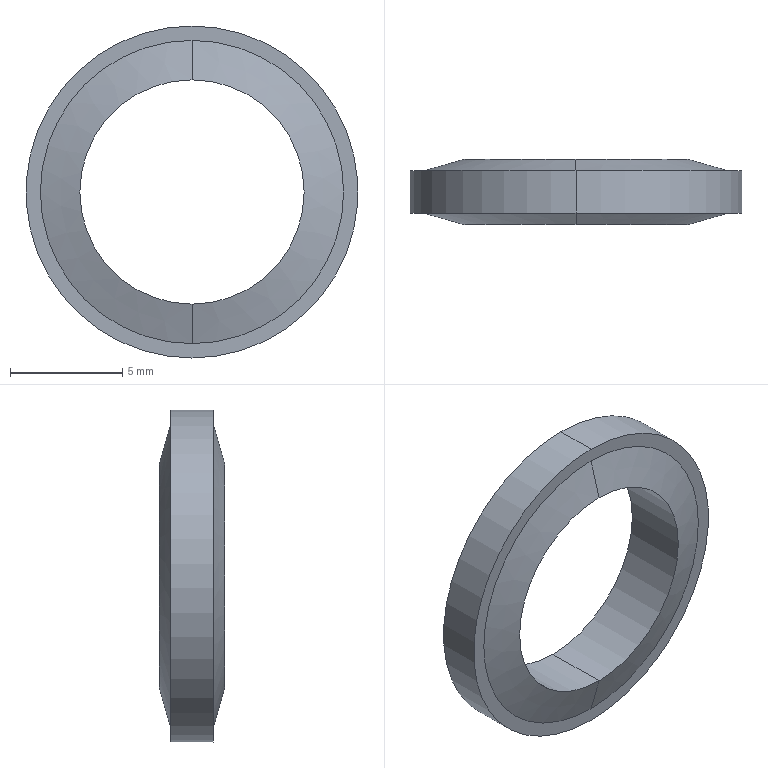Part | SolidWorks | features BaseBody 2 | 2 solids | 14 faces | box 14.8 x 2.9 x 14.8 mm | volume 208.528 mm3 | cylinder 8 | cone 4 | plane 2 | commonest cylinder face diameters 13.52 x4 10 x2 14.8 x2
STEP:
#1=CARTESIAN_POINT('',(0.,1.9,-6.76));
#2=VERTEX_POINT('',#1);
#3=CARTESIAN_POINT('',(0.,0.,-6.76));
#4=VERTEX_POINT('',#3);
#5=CARTESIAN_POINT('',(0.,1.9,-6.76));
#6=DIRECTION('',(0.,-1.,0.));
#7=VECTOR('',#6,1000.);
#8=LINE('',#5,#7);
#9=EDGE_CURVE('',#2,#4,#8,.T.);
#10=ORIENTED_EDGE('',*,*,#9,.T.);
#11=CARTESIAN_POINT('',(0.,0.,6.76));
#12=VERTEX_POINT('',#11);
#13=CARTESIAN_POINT('',(0.,0.,0.));
#14=DIRECTION('',(0.,-1.,0.));
#15=DIRECTION('',(0.,0.,-1.));
#16=AXIS2_PLACEMENT_3D('',#13,#14,#15);
#17=CIRCLE('',#16,6.76);
#18=EDGE_CURVE('',#4,#12,#17,.T.);
#19=ORIENTED_EDGE('',*,*,#18,.T.);
#20=CARTESIAN_POINT('',(0.,1.9,6.76));
#21=VERTEX_POINT('',#20);
#22=CARTESIAN_POINT('',(0.,1.9,6.76));
#23=DIRECTION('',(0.,-1.,0.));
#24=VECTOR('',#23,1000.);
#25=LINE('',#22,#24);
#26=EDGE_CURVE('',#21,#12,#25,.T.);
#27=ORIENTED_EDGE('',*,*,#26,.F.);
#28=CARTESIAN_POINT('',(0.,1.9,0.));
#29=DIRECTION('',(0.,-1.,0.));
#30=DIRECTION('',(0.,0.,-1.));
#31=AXIS2_PLACEMENT_3D('',#28,#29,#30);
#32=CIRCLE('',#31,6.76);
#33=EDGE_CURVE('',#2,#21,#32,.T.);
#34=ORIENTED_EDGE('',*,*,#33,.F.);
#35=EDGE_LOOP('',(#10,#19,#27,#34));
#36=FACE_OUTER_BOUND('',#35,.T.);
#37=CARTESIAN_POINT('',(0.,1.9,0.));
#38=DIRECTION('',(0.,-1.,0.));
#39=DIRECTION('',(0.,0.,1.));
#40=AXIS2_PLACEMENT_3D('',#37,#38,#39);
#41=CYLINDRICAL_SURFACE('',#40,6.76);
#42=ADVANCED_FACE('',(#36),#41,.F.);
#43=CARTESIAN_POINT('',(0.,1.9,-7.4));
#44=VERTEX_POINT('',#43);
#45=CARTESIAN_POINT('',(0.,0.,-7.4));
#46=VERTEX_POINT('',#45);
#47=CARTESIAN_POINT('',(0.,1.9,-7.4));
#48=DIRECTION('',(0.,-1.,0.));
#49=VECTOR('',#48,1000.);
#50=LINE('',#47,#49);
#51=EDGE_CURVE('',#44,#46,#50,.T.);
#52=ORIENTED_EDGE('',*,*,#51,.T.);
#53=CARTESIAN_POINT('',(0.,0.,7.4));
#54=VERTEX_POINT('',#53);
#55=CARTESIAN_POINT('',(0.,0.,0.));
#56=DIRECTION('',(0.,-1.,0.));
#57=DIRECTION('',(0.,0.,-1.));
#58=AXIS2_PLACEMENT_3D('',#55,#56,#57);
#59=CIRCLE('',#58,7.4);
#60=EDGE_CURVE('',#54,#46,#59,.T.);
#61=ORIENTED_EDGE('',*,*,#60,.F.);
#62=CARTESIAN_POINT('',(0.,1.9,7.4));
#63=VERTEX_POINT('',#62);
#64=CARTESIAN_POINT('',(0.,1.9,7.4));
#65=DIRECTION('',(0.,-1.,0.));
#66=VECTOR('',#65,1000.);
#67=LINE('',#64,#66);
#68=EDGE_CURVE('',#63,#54,#67,.T.);
#69=ORIENTED_EDGE('',*,*,#68,.F.);
#70=CARTESIAN_POINT('',(0.,1.9,0.));
#71=DIRECTION('',(0.,-1.,0.));
#72=DIRECTION('',(0.,0.,-1.));
#73=AXIS2_PLACEMENT_3D('',#70,#71,#72);
#74=CIRCLE('',#73,7.4);
#75=EDGE_CURVE('',#63,#44,#74,.T.);
#76=ORIENTED_EDGE('',*,*,#75,.T.);
#77=EDGE_LOOP('',(#52,#61,#69,#76));
#78=FACE_OUTER_BOUND('',#77,.T.);
#79=CARTESIAN_POINT('',(0.,1.9,0.));
#80=DIRECTION('',(0.,-1.,0.));
#81=DIRECTION('',(0.,0.,1.));
#82=AXIS2_PLACEMENT_3D('',#79,#80,#81);
#83=CYLINDRICAL_SURFACE('',#82,7.4);
#84=ADVANCED_FACE('',(#78),#83,.T.);
#85=CARTESIAN_POINT('',(0.,0.,0.));
#86=DIRECTION('',(0.,-1.,0.));
#87=DIRECTION('',(0.,0.,-1.));
#88=AXIS2_PLACEMENT_3D('',#85,#86,#87);
#89=CIRCLE('',#88,6.76);
#90=EDGE_CURVE('',#12,#4,#89,.T.);
#91=ORIENTED_EDGE('',*,*,#90,.F.);
#92=ORIENTED_EDGE('',*,*,#18,.F.);
#93=EDGE_LOOP('',(#91,#92));
#94=FACE_BOUND('',#93,.T.);
#95=ORIENTED_EDGE('',*,*,#60,.T.);
#96=CARTESIAN_POINT('',(0.,0.,0.));
#97=DIRECTION('',(0.,-1.,0.));
#98=DIRECTION('',(0.,0.,-1.));
#99=AXIS2_PLACEMENT_3D('',#96,#97,#98);
#100=CIRCLE('',#99,7.4);
#101=EDGE_CURVE('',#46,#54,#100,.T.);
#102=ORIENTED_EDGE('',*,*,#101,.T.);
#103=EDGE_LOOP('',(#95,#102));
#104=FACE_OUTER_BOUND('',#103,.T.);
#105=CARTESIAN_POINT('',(0.,0.,0.));
#106=DIRECTION('',(0.,1.,0.));
#107=DIRECTION('',(1.,0.,0.));
#108=AXIS2_PLACEMENT_3D('',#105,#106,#107);
#109=PLANE('',#108);
#110=ADVANCED_FACE('',(#94,#104),#109,.F.);
#111=CARTESIAN_POINT('',(0.,1.9,0.));
#112=DIRECTION('',(0.,-1.,0.));
#113=DIRECTION('',(0.,0.,-1.));
#114=AXIS2_PLACEMENT_3D('',#111,#112,#113);
#115=CIRCLE('',#114,6.76);
#116=EDGE_CURVE('',#21,#2,#115,.T.);
#117=ORIENTED_EDGE('',*,*,#116,.T.);
#118=ORIENTED_EDGE('',*,*,#33,.T.);
#119=EDGE_LOOP('',(#117,#118));
#120=FACE_BOUND('',#119,.T.);
#121=ORIENTED_EDGE('',*,*,#75,.F.);
#122=CARTESIAN_POINT('',(0.,1.9,0.));
#123=DIRECTION('',(0.,-1.,0.));
#124=DIRECTION('',(0.,0.,-1.));
#125=AXIS2_PLACEMENT_3D('',#122,#123,#124);
#126=CIRCLE('',#125,7.4);
#127=EDGE_CURVE('',#44,#63,#126,.T.);
#128=ORIENTED_EDGE('',*,*,#127,.F.);
#129=EDGE_LOOP('',(#121,#128));
#130=FACE_OUTER_BOUND('',#129,.T.);
#131=CARTESIAN_POINT('',(0.,1.9,0.));
#132=DIRECTION('',(0.,1.,0.));
#133=DIRECTION('',(1.,0.,0.));
#134=AXIS2_PLACEMENT_3D('',#131,#132,#133);
#135=PLANE('',#134);
#136=ADVANCED_FACE('',(#120,#130),#135,.T.);
#137=ORIENTED_EDGE('',*,*,#127,.T.);
#138=ORIENTED_EDGE('',*,*,#68,.T.);
#139=ORIENTED_EDGE('',*,*,#101,.F.);
#140=ORIENTED_EDGE('',*,*,#51,.F.);
#141=EDGE_LOOP('',(#137,#138,#139,#140));
#142=FACE_OUTER_BOUND('',#141,.T.);
#143=CARTESIAN_POINT('',(0.,1.9,0.));
#144=DIRECTION('',(0.,-1.,0.));
#145=DIRECTION('',(0.,0.,1.));
#146=AXIS2_PLACEMENT_3D('',#143,#144,#145);
#147=CYLINDRICAL_SURFACE('',#146,7.4);
#148=ADVANCED_FACE('',(#142),#147,.T.);
#149=ORIENTED_EDGE('',*,*,#116,.F.);
#150=ORIENTED_EDGE('',*,*,#26,.T.);
#151=ORIENTED_EDGE('',*,*,#90,.T.);
#152=ORIENTED_EDGE('',*,*,#9,.F.);
#153=EDGE_LOOP('',(#149,#150,#151,#152));
#154=FACE_OUTER_BOUND('',#153,.T.);
#155=CARTESIAN_POINT('',(0.,1.9,0.));
#156=DIRECTION('',(0.,-1.,0.));
#157=DIRECTION('',(0.,0.,1.));
#158=AXIS2_PLACEMENT_3D('',#155,#156,#157);
#159=CYLINDRICAL_SURFACE('',#158,6.76);
#160=ADVANCED_FACE('',(#154),#159,.F.);
#161=CLOSED_SHELL('',(#42,#84,#110,#136,#148,#160));
#162=MANIFOLD_SOLID_BREP('',#161);
#163=CARTESIAN_POINT('',(0.,2.4,-5.));
#164=VERTEX_POINT('',#163);
#165=CARTESIAN_POINT('',(0.,-0.5,-5.));
#166=VERTEX_POINT('',#165);
#167=CARTESIAN_POINT('',(0.,0.,-5.));
#168=DIRECTION('',(0.,-1.,0.));
#169=VECTOR('',#168,1000.);
#170=LINE('',#167,#169);
#171=EDGE_CURVE('',#164,#166,#170,.T.);
#172=ORIENTED_EDGE('',*,*,#171,.T.);
#173=CARTESIAN_POINT('',(0.,-0.5,5.));
#174=VERTEX_POINT('',#173);
#175=CARTESIAN_POINT('',(0.,-0.5,0.));
#176=DIRECTION('',(0.,1.,0.));
#177=DIRECTION('',(0.,0.,1.));
#178=AXIS2_PLACEMENT_3D('',#175,#176,#177);
#179=CIRCLE('',#178,5.);
#180=EDGE_CURVE('',#174,#166,#179,.T.);
#181=ORIENTED_EDGE('',*,*,#180,.F.);
#182=CARTESIAN_POINT('',(0.,2.4,5.));
#183=VERTEX_POINT('',#182);
#184=CARTESIAN_POINT('',(0.,0.,5.));
#185=DIRECTION('',(0.,-1.,0.));
#186=VECTOR('',#185,1000.);
#187=LINE('',#184,#186);
#188=EDGE_CURVE('',#183,#174,#187,.T.);
#189=ORIENTED_EDGE('',*,*,#188,.F.);
#190=CARTESIAN_POINT('',(0.,2.4,0.));
#191=DIRECTION('',(0.,1.,0.));
#192=DIRECTION('',(0.,0.,1.));
#193=AXIS2_PLACEMENT_3D('',#190,#191,#192);
#194=CIRCLE('',#193,5.);
#195=EDGE_CURVE('',#183,#164,#194,.T.);
#196=ORIENTED_EDGE('',*,*,#195,.T.);
#197=EDGE_LOOP('',(#172,#181,#189,#196));
#198=FACE_OUTER_BOUND('',#197,.T.);
#199=CARTESIAN_POINT('',(0.,0.,0.));
#200=DIRECTION('',(0.,-1.,0.));
#201=DIRECTION('',(0.,0.,1.));
#202=AXIS2_PLACEMENT_3D('',#199,#200,#201);
#203=CYLINDRICAL_SURFACE('',#202,5.);
#204=ADVANCED_FACE('',(#198),#203,.F.);
#205=CARTESIAN_POINT('',(0.,0.,6.76));
#206=VERTEX_POINT('',#205);
#207=CARTESIAN_POINT('',(0.,-0.5,5.));
#208=DIRECTION('',(0.,0.2733,0.9619));
#209=VECTOR('',#208,1000.);
#210=LINE('',#207,#209);
#211=EDGE_CURVE('',#174,#206,#210,.T.);
#212=ORIENTED_EDGE('',*,*,#211,.T.);
#213=CARTESIAN_POINT('',(0.,0.,-6.76));
#214=VERTEX_POINT('',#213);
#215=CARTESIAN_POINT('',(0.,0.,0.));
#216=DIRECTION('',(0.,1.,0.));
#217=DIRECTION('',(0.,0.,1.));
#218=AXIS2_PLACEMENT_3D('',#215,#216,#217);
#219=CIRCLE('',#218,6.76);
#220=EDGE_CURVE('',#214,#206,#219,.T.);
#221=ORIENTED_EDGE('',*,*,#220,.F.);
#222=CARTESIAN_POINT('',(0.,-0.5,-5.));
#223=DIRECTION('',(0.,0.2733,-0.9619));
#224=VECTOR('',#223,1000.);
#225=LINE('',#222,#224);
#226=EDGE_CURVE('',#166,#214,#225,.T.);
#227=ORIENTED_EDGE('',*,*,#226,.F.);
#228=CARTESIAN_POINT('',(0.,-0.5,0.));
#229=DIRECTION('',(0.,1.,0.));
#230=DIRECTION('',(0.,0.,1.));
#231=AXIS2_PLACEMENT_3D('',#228,#229,#230);
#232=CIRCLE('',#231,5.);
#233=EDGE_CURVE('',#166,#174,#232,.T.);
#234=ORIENTED_EDGE('',*,*,#233,.T.);
#235=EDGE_LOOP('',(#212,#221,#227,#234));
#236=FACE_OUTER_BOUND('',#235,.T.);
#237=CARTESIAN_POINT('',(0.,-0.5,0.));
#238=DIRECTION('',(0.,1.,0.));
#239=DIRECTION('',(0.,0.,-1.));
#240=AXIS2_PLACEMENT_3D('',#237,#238,#239);
#241=CONICAL_SURFACE('',#240,5.,1.294);
#242=ADVANCED_FACE('',(#236),#241,.T.);
#243=CARTESIAN_POINT('',(0.,1.9,-6.76));
#244=VERTEX_POINT('',#243);
#245=CARTESIAN_POINT('',(0.,0.,-6.76));
#246=DIRECTION('',(0.,-1.,0.));
#247=VECTOR('',#246,1000.);
#248=LINE('',#245,#247);
#249=EDGE_CURVE('',#244,#214,#248,.T.);
#250=ORIENTED_EDGE('',*,*,#249,.T.);
#251=ORIENTED_EDGE('',*,*,#220,.T.);
#252=CARTESIAN_POINT('',(0.,1.9,6.76));
#253=VERTEX_POINT('',#252);
#254=CARTESIAN_POINT('',(0.,0.,6.76));
#255=DIRECTION('',(0.,-1.,0.));
#256=VECTOR('',#255,1000.);
#257=LINE('',#254,#256);
#258=EDGE_CURVE('',#253,#206,#257,.T.);
#259=ORIENTED_EDGE('',*,*,#258,.F.);
#260=CARTESIAN_POINT('',(0.,1.9,0.));
#261=DIRECTION('',(0.,1.,0.));
#262=DIRECTION('',(0.,0.,1.));
#263=AXIS2_PLACEMENT_3D('',#260,#261,#262);
#264=CIRCLE('',#263,6.76);
#265=EDGE_CURVE('',#244,#253,#264,.T.);
#266=ORIENTED_EDGE('',*,*,#265,.F.);
#267=EDGE_LOOP('',(#250,#251,#259,#266));
#268=FACE_OUTER_BOUND('',#267,.T.);
#269=CARTESIAN_POINT('',(0.,0.,0.));
#270=DIRECTION('',(0.,-1.,0.));
#271=DIRECTION('',(0.,0.,1.));
#272=AXIS2_PLACEMENT_3D('',#269,#270,#271);
#273=CYLINDRICAL_SURFACE('',#272,6.76);
#274=ADVANCED_FACE('',(#268),#273,.T.);
#275=CARTESIAN_POINT('',(0.,1.9,-6.76));
#276=DIRECTION('',(0.,-0.2733,-0.9619));
#277=VECTOR('',#276,1000.);
#278=LINE('',#275,#277);
#279=EDGE_CURVE('',#164,#244,#278,.T.);
#280=ORIENTED_EDGE('',*,*,#279,.T.);
#281=ORIENTED_EDGE('',*,*,#265,.T.);
#282=CARTESIAN_POINT('',(0.,1.9,6.76));
#283=DIRECTION('',(0.,-0.2733,0.9619));
#284=VECTOR('',#283,1000.);
#285=LINE('',#282,#284);
#286=EDGE_CURVE('',#183,#253,#285,.T.);
#287=ORIENTED_EDGE('',*,*,#286,.F.);
#288=CARTESIAN_POINT('',(0.,2.4,0.));
#289=DIRECTION('',(0.,1.,0.));
#290=DIRECTION('',(0.,0.,1.));
#291=AXIS2_PLACEMENT_3D('',#288,#289,#290);
#292=CIRCLE('',#291,5.);
#293=EDGE_CURVE('',#164,#183,#292,.T.);
#294=ORIENTED_EDGE('',*,*,#293,.F.);
#295=EDGE_LOOP('',(#280,#281,#287,#294));
#296=FACE_OUTER_BOUND('',#295,.T.);
#297=CARTESIAN_POINT('',(0.,1.9,0.));
#298=DIRECTION('',(0.,-1.,0.));
#299=DIRECTION('',(0.,0.,1.));
#300=AXIS2_PLACEMENT_3D('',#297,#298,#299);
#301=CONICAL_SURFACE('',#300,6.76,1.294);
#302=ADVANCED_FACE('',(#296),#301,.T.);
#303=ORIENTED_EDGE('',*,*,#195,.F.);
#304=ORIENTED_EDGE('',*,*,#286,.T.);
#305=CARTESIAN_POINT('',(0.,1.9,0.));
#306=DIRECTION('',(0.,1.,0.));
#307=DIRECTION('',(0.,0.,1.));
#308=AXIS2_PLACEMENT_3D('',#305,#306,#307);
#309=CIRCLE('',#308,6.76);
#310=EDGE_CURVE('',#253,#244,#309,.T.);
#311=ORIENTED_EDGE('',*,*,#310,.T.);
#312=ORIENTED_EDGE('',*,*,#279,.F.);
#313=EDGE_LOOP('',(#303,#304,#311,#312));
#314=FACE_OUTER_BOUND('',#313,.T.);
#315=CARTESIAN_POINT('',(0.,1.9,0.));
#316=DIRECTION('',(0.,-1.,0.));
#317=DIRECTION('',(0.,0.,1.));
#318=AXIS2_PLACEMENT_3D('',#315,#316,#317);
#319=CONICAL_SURFACE('',#318,6.76,1.294);
#320=ADVANCED_FACE('',(#314),#319,.T.);
#321=ORIENTED_EDGE('',*,*,#310,.F.);
#322=ORIENTED_EDGE('',*,*,#258,.T.);
#323=CARTESIAN_POINT('',(0.,0.,0.));
#324=DIRECTION('',(0.,1.,0.));
#325=DIRECTION('',(0.,0.,1.));
#326=AXIS2_PLACEMENT_3D('',#323,#324,#325);
#327=CIRCLE('',#326,6.76);
#328=EDGE_CURVE('',#206,#214,#327,.T.);
#329=ORIENTED_EDGE('',*,*,#328,.T.);
#330=ORIENTED_EDGE('',*,*,#249,.F.);
#331=EDGE_LOOP('',(#321,#322,#329,#330));
#332=FACE_OUTER_BOUND('',#331,.T.);
#333=CARTESIAN_POINT('',(0.,0.,0.));
#334=DIRECTION('',(0.,-1.,0.));
#335=DIRECTION('',(0.,0.,1.));
#336=AXIS2_PLACEMENT_3D('',#333,#334,#335);
#337=CYLINDRICAL_SURFACE('',#336,6.76);
#338=ADVANCED_FACE('',(#332),#337,.T.);
#339=ORIENTED_EDGE('',*,*,#180,.T.);
#340=ORIENTED_EDGE('',*,*,#226,.T.);
#341=ORIENTED_EDGE('',*,*,#328,.F.);
#342=ORIENTED_EDGE('',*,*,#211,.F.);
#343=EDGE_LOOP('',(#339,#340,#341,#342));
#344=FACE_OUTER_BOUND('',#343,.T.);
#345=CARTESIAN_POINT('',(0.,-0.5,0.));
#346=DIRECTION('',(0.,1.,0.));
#347=DIRECTION('',(0.,0.,-1.));
#348=AXIS2_PLACEMENT_3D('',#345,#346,#347);
#349=CONICAL_SURFACE('',#348,5.,1.294);
#350=ADVANCED_FACE('',(#344),#349,.T.);
#351=ORIENTED_EDGE('',*,*,#293,.T.);
#352=ORIENTED_EDGE('',*,*,#188,.T.);
#353=ORIENTED_EDGE('',*,*,#233,.F.);
#354=ORIENTED_EDGE('',*,*,#171,.F.);
#355=EDGE_LOOP('',(#351,#352,#353,#354));
#356=FACE_OUTER_BOUND('',#355,.T.);
#357=CARTESIAN_POINT('',(0.,0.,0.));
#358=DIRECTION('',(0.,-1.,0.));
#359=DIRECTION('',(0.,0.,1.));
#360=AXIS2_PLACEMENT_3D('',#357,#358,#359);
#361=CYLINDRICAL_SURFACE('',#360,5.);
#362=ADVANCED_FACE('',(#356),#361,.F.);
#363=CLOSED_SHELL('',(#204,#242,#274,#302,#320,#338,#350,#362));
#364=MANIFOLD_SOLID_BREP('',#363);
#365=CARTESIAN_POINT('',(0.,0.,0.));
#366=DIRECTION('',(0.,0.,1.));
#367=DIRECTION('',(1.,0.,0.));
#368=AXIS2_PLACEMENT_3D('',#365,#366,#367);
#369=(LENGTH_UNIT()NAMED_UNIT(*)SI_UNIT(.MILLI.,.METRE.));
#370=UNCERTAINTY_MEASURE_WITH_UNIT(LENGTH_MEASURE(0.00001),#369,'','');
#371=(NAMED_UNIT(*)PLANE_ANGLE_UNIT()SI_UNIT($,.RADIAN.));
#372=(NAMED_UNIT(*)SI_UNIT($,.STERADIAN.)SOLID_ANGLE_UNIT());
#373=(GEOMETRIC_REPRESENTATION_CONTEXT(3)GLOBAL_UNCERTAINTY_ASSIGNED_CONTEXT((#370))GLOBAL_UNIT_ASSIGNED_CONTEXT((#369,#371,#372))REPRESENTATION_CONTEXT('',''));
#374=ADVANCED_BREP_SHAPE_REPRESENTATION('',(#162,#364,#368),#373);